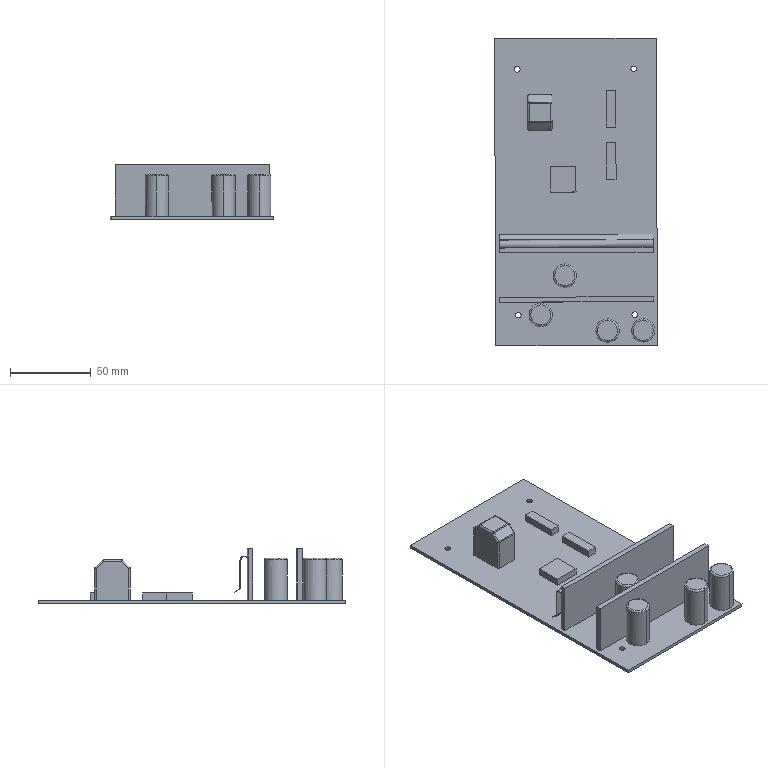Part | SolidWorks | features BaseBody 1 | 1 solid | 100 faces | box 100.826 x 190.433 x 34 mm | volume 83703 mm3 | plane 48 | cylinder 36 | spline 16 | commonest cylinder face diameters 2 x16 3.5 x8 14.35 x8 2.418 x1 2.818 x1 4.553 x1